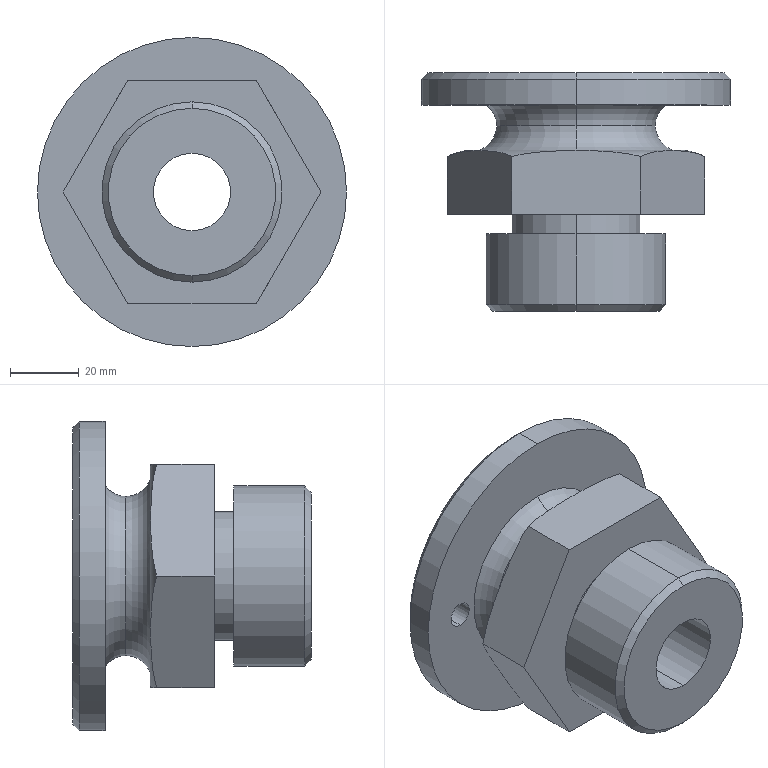Part | SolidWorks | features Chamfer 2, ICE 2, RevCut 1, Revolution 1, Scale 1 | 1 solid | 34 faces | box 90 x 69.375 x 90 mm | volume 178103 mm3 | cylinder 12 | plane 12 | torus 6 | cone 4 | commonest cylinder face diameters 7.5 x4 22.5 x2 37.5 x2 52.5 x2 90 x2
STEP:
#1=CARTESIAN_POINT('',(0.,27.536,-28.125));
#2=VERTEX_POINT('',#1);
#3=CARTESIAN_POINT('',(0.,34.594,-23.16));
#4=VERTEX_POINT('',#3);
#5=CARTESIAN_POINT('',(0.,34.594,-30.66));
#6=DIRECTION('',(-1.,0.,0.));
#7=DIRECTION('',(0.,0.,1.));
#8=AXIS2_PLACEMENT_3D('',#5,#6,#7);
#9=CIRCLE('',#8,7.5);
#10=EDGE_CURVE('',#2,#4,#9,.T.);
#11=ORIENTED_EDGE('',*,*,#10,.T.);
#12=CARTESIAN_POINT('',(0.,34.594,23.16));
#13=VERTEX_POINT('',#12);
#14=CARTESIAN_POINT('',(0.,34.594,-0.000000001));
#15=DIRECTION('',(0.,-1.,0.));
#16=DIRECTION('',(0.,0.,-1.));
#17=AXIS2_PLACEMENT_3D('',#14,#15,#16);
#18=CIRCLE('',#17,23.16);
#19=EDGE_CURVE('',#4,#13,#18,.T.);
#20=ORIENTED_EDGE('',*,*,#19,.T.);
#21=CARTESIAN_POINT('',(0.,27.536,28.125));
#22=VERTEX_POINT('',#21);
#23=CARTESIAN_POINT('',(0.,34.594,30.66));
#24=DIRECTION('',(1.,0.,0.));
#25=DIRECTION('',(0.,0.,-1.));
#26=AXIS2_PLACEMENT_3D('',#23,#24,#25);
#27=CIRCLE('',#26,7.5);
#28=EDGE_CURVE('',#22,#13,#27,.T.);
#29=ORIENTED_EDGE('',*,*,#28,.F.);
#30=CARTESIAN_POINT('',(0.,27.536,-0.000000001));
#31=DIRECTION('',(0.,-1.,0.));
#32=DIRECTION('',(0.,0.,-1.));
#33=AXIS2_PLACEMENT_3D('',#30,#31,#32);
#34=CIRCLE('',#33,28.125);
#35=EDGE_CURVE('',#2,#22,#34,.T.);
#36=ORIENTED_EDGE('',*,*,#35,.F.);
#37=EDGE_LOOP('',(#11,#20,#29,#36));
#38=FACE_OUTER_BOUND('',#37,.T.);
#39=CARTESIAN_POINT('',(0.,34.594,-0.000000001));
#40=DIRECTION('',(0.,-1.,0.));
#41=DIRECTION('',(0.,0.,-1.));
#42=AXIS2_PLACEMENT_3D('',#39,#40,#41);
#43=TOROIDAL_SURFACE('',#42,30.66,7.5);
#44=ADVANCED_FACE('',(#38),#43,.F.);
#45=ORIENTED_EDGE('',*,*,#28,.T.);
#46=CARTESIAN_POINT('',(0.,34.594,-0.000000001));
#47=DIRECTION('',(0.,-1.,0.));
#48=DIRECTION('',(0.,0.,-1.));
#49=AXIS2_PLACEMENT_3D('',#46,#47,#48);
#50=CIRCLE('',#49,23.16);
#51=EDGE_CURVE('',#13,#4,#50,.T.);
#52=ORIENTED_EDGE('',*,*,#51,.T.);
#53=ORIENTED_EDGE('',*,*,#10,.F.);
#54=CARTESIAN_POINT('',(0.,27.536,-0.000000001));
#55=DIRECTION('',(0.,-1.,0.));
#56=DIRECTION('',(0.,0.,-1.));
#57=AXIS2_PLACEMENT_3D('',#54,#55,#56);
#58=CIRCLE('',#57,28.125);
#59=EDGE_CURVE('',#22,#2,#58,.T.);
#60=ORIENTED_EDGE('',*,*,#59,.F.);
#61=EDGE_LOOP('',(#45,#52,#53,#60));
#62=FACE_OUTER_BOUND('',#61,.T.);
#63=CARTESIAN_POINT('',(0.,34.594,-0.000000001));
#64=DIRECTION('',(0.,-1.,0.));
#65=DIRECTION('',(0.,0.,-1.));
#66=AXIS2_PLACEMENT_3D('',#63,#64,#65);
#67=TOROIDAL_SURFACE('',#66,30.66,7.5);
#68=ADVANCED_FACE('',(#62),#67,.F.);
#69=CARTESIAN_POINT('',(-31.875,40.661,-3.75));
#70=VERTEX_POINT('',#69);
#71=CARTESIAN_POINT('',(-31.875,40.661,3.75));
#72=VERTEX_POINT('',#71);
#73=CARTESIAN_POINT('',(-31.875,40.661,-0.000000001));
#74=DIRECTION('',(0.,1.,0.));
#75=DIRECTION('',(0.,0.,-1.));
#76=AXIS2_PLACEMENT_3D('',#73,#74,#75);
#77=CIRCLE('',#76,3.75);
#78=EDGE_CURVE('',#70,#72,#77,.T.);
#79=ORIENTED_EDGE('',*,*,#78,.F.);
#80=CARTESIAN_POINT('',(-31.875,50.036,-3.75));
#81=VERTEX_POINT('',#80);
#82=CARTESIAN_POINT('',(-31.875,-19.341,-3.75));
#83=DIRECTION('',(0.,1.,0.));
#84=VECTOR('',#83,1000.);
#85=LINE('',#82,#84);
#86=EDGE_CURVE('',#70,#81,#85,.T.);
#87=ORIENTED_EDGE('',*,*,#86,.T.);
#88=CARTESIAN_POINT('',(-31.875,50.036,3.75));
#89=VERTEX_POINT('',#88);
#90=CARTESIAN_POINT('',(-31.875,50.036,-0.000000001));
#91=DIRECTION('',(0.,1.,0.));
#92=DIRECTION('',(0.,0.,-1.));
#93=AXIS2_PLACEMENT_3D('',#90,#91,#92);
#94=CIRCLE('',#93,3.75);
#95=EDGE_CURVE('',#81,#89,#94,.T.);
#96=ORIENTED_EDGE('',*,*,#95,.T.);
#97=CARTESIAN_POINT('',(-31.875,-19.341,3.75));
#98=DIRECTION('',(0.,1.,0.));
#99=VECTOR('',#98,1000.);
#100=LINE('',#97,#99);
#101=EDGE_CURVE('',#72,#89,#100,.T.);
#102=ORIENTED_EDGE('',*,*,#101,.F.);
#103=EDGE_LOOP('',(#79,#87,#96,#102));
#104=FACE_OUTER_BOUND('',#103,.T.);
#105=CARTESIAN_POINT('',(-31.875,-19.341,-0.000000001));
#106=DIRECTION('',(0.,1.,0.));
#107=DIRECTION('',(0.,0.,1.));
#108=AXIS2_PLACEMENT_3D('',#105,#106,#107);
#109=CYLINDRICAL_SURFACE('',#108,3.75);
#110=ADVANCED_FACE('',(#104),#109,.F.);
#111=CARTESIAN_POINT('',(31.875,40.661,-3.75));
#112=VERTEX_POINT('',#111);
#113=CARTESIAN_POINT('',(31.875,40.661,3.75));
#114=VERTEX_POINT('',#113);
#115=CARTESIAN_POINT('',(31.875,40.661,-0.000000001));
#116=DIRECTION('',(0.,1.,0.));
#117=DIRECTION('',(0.,0.,-1.));
#118=AXIS2_PLACEMENT_3D('',#115,#116,#117);
#119=CIRCLE('',#118,3.75);
#120=EDGE_CURVE('',#112,#114,#119,.T.);
#121=ORIENTED_EDGE('',*,*,#120,.F.);
#122=CARTESIAN_POINT('',(31.875,50.036,-3.75));
#123=VERTEX_POINT('',#122);
#124=CARTESIAN_POINT('',(31.875,-19.341,-3.75));
#125=DIRECTION('',(0.,1.,0.));
#126=VECTOR('',#125,1000.);
#127=LINE('',#124,#126);
#128=EDGE_CURVE('',#112,#123,#127,.T.);
#129=ORIENTED_EDGE('',*,*,#128,.T.);
#130=CARTESIAN_POINT('',(31.875,50.036,3.75));
#131=VERTEX_POINT('',#130);
#132=CARTESIAN_POINT('',(31.875,50.036,-0.000000001));
#133=DIRECTION('',(0.,1.,0.));
#134=DIRECTION('',(0.,0.,1.));
#135=AXIS2_PLACEMENT_3D('',#132,#133,#134);
#136=CIRCLE('',#135,3.75);
#137=EDGE_CURVE('',#123,#131,#136,.T.);
#138=ORIENTED_EDGE('',*,*,#137,.T.);
#139=CARTESIAN_POINT('',(31.875,-19.341,3.75));
#140=DIRECTION('',(0.,1.,0.));
#141=VECTOR('',#140,1000.);
#142=LINE('',#139,#141);
#143=EDGE_CURVE('',#114,#131,#142,.T.);
#144=ORIENTED_EDGE('',*,*,#143,.F.);
#145=EDGE_LOOP('',(#121,#129,#138,#144));
#146=FACE_OUTER_BOUND('',#145,.T.);
#147=CARTESIAN_POINT('',(31.875,-19.341,-0.000000001));
#148=DIRECTION('',(0.,1.,0.));
#149=DIRECTION('',(0.,0.,1.));
#150=AXIS2_PLACEMENT_3D('',#147,#148,#149);
#151=CYLINDRICAL_SURFACE('',#150,3.75);
#152=ADVANCED_FACE('',(#146),#151,.F.);
#153=CARTESIAN_POINT('',(0.,50.036,43.125));
#154=VERTEX_POINT('',#153);
#155=CARTESIAN_POINT('',(0.,50.036,-43.125));
#156=VERTEX_POINT('',#155);
#157=CARTESIAN_POINT('',(0.,50.036,-0.000000001));
#158=DIRECTION('',(0.,1.,0.));
#159=DIRECTION('',(0.,0.,1.));
#160=AXIS2_PLACEMENT_3D('',#157,#158,#159);
#161=CIRCLE('',#160,43.125);
#162=EDGE_CURVE('',#154,#156,#161,.T.);
#163=ORIENTED_EDGE('',*,*,#162,.F.);
#164=CARTESIAN_POINT('',(0.,48.161,45.));
#165=VERTEX_POINT('',#164);
#166=CARTESIAN_POINT('',(0.,48.161,45.));
#167=DIRECTION('',(0.,-0.7071,0.7071));
#168=VECTOR('',#167,1000.);
#169=LINE('',#166,#168);
#170=EDGE_CURVE('',#154,#165,#169,.T.);
#171=ORIENTED_EDGE('',*,*,#170,.T.);
#172=CARTESIAN_POINT('',(0.,48.161,-45.));
#173=VERTEX_POINT('',#172);
#174=CARTESIAN_POINT('',(0.,48.161,-0.000000001));
#175=DIRECTION('',(0.,-1.,0.));
#176=DIRECTION('',(0.,0.,1.));
#177=AXIS2_PLACEMENT_3D('',#174,#175,#176);
#178=CIRCLE('',#177,45.);
#179=EDGE_CURVE('',#173,#165,#178,.T.);
#180=ORIENTED_EDGE('',*,*,#179,.F.);
#181=CARTESIAN_POINT('',(0.,48.161,-45.));
#182=DIRECTION('',(0.,-0.7071,-0.7071));
#183=VECTOR('',#182,1000.);
#184=LINE('',#181,#183);
#185=EDGE_CURVE('',#156,#173,#184,.T.);
#186=ORIENTED_EDGE('',*,*,#185,.F.);
#187=EDGE_LOOP('',(#163,#171,#180,#186));
#188=FACE_OUTER_BOUND('',#187,.T.);
#189=CARTESIAN_POINT('',(0.,48.161,-0.000000001));
#190=DIRECTION('',(0.,-1.,0.));
#191=DIRECTION('',(0.,0.,-1.));
#192=AXIS2_PLACEMENT_3D('',#189,#190,#191);
#193=CONICAL_SURFACE('',#192,45.,0.7854);
#194=ADVANCED_FACE('',(#188),#193,.T.);
#195=CARTESIAN_POINT('',(0.,27.536,-31.152));
#196=VERTEX_POINT('',#195);
#197=CARTESIAN_POINT('',(0.,27.536,31.152));
#198=VERTEX_POINT('',#197);
#199=CARTESIAN_POINT('',(0.,27.536,-0.000000001));
#200=DIRECTION('',(0.,-1.,0.));
#201=DIRECTION('',(0.,0.,-1.));
#202=AXIS2_PLACEMENT_3D('',#199,#200,#201);
#203=CIRCLE('',#202,31.152);
#204=EDGE_CURVE('',#196,#198,#203,.T.);
#205=ORIENTED_EDGE('',*,*,#204,.T.);
#206=CARTESIAN_POINT('',(0.,27.363,32.476));
#207=VERTEX_POINT('',#206);
#208=CARTESIAN_POINT('',(0.,10.729,29.639));
#209=DIRECTION('',(1.,0.,0.));
#210=DIRECTION('',(0.,0.,-1.));
#211=AXIS2_PLACEMENT_3D('',#208,#209,#210);
#212=CIRCLE('',#211,16.875);
#213=EDGE_CURVE('',#198,#207,#212,.T.);
#214=ORIENTED_EDGE('',*,*,#213,.T.);
#215=CARTESIAN_POINT('',(18.75,25.661,32.476));
#216=VERTEX_POINT('',#215);
#217=CARTESIAN_POINT('',(18.75,25.661,32.476));
#218=CARTESIAN_POINT('',(17.221,26.063,32.476));
#219=CARTESIAN_POINT('',(15.679,26.359,32.476));
#220=CARTESIAN_POINT('',(12.575,26.81,32.476));
#221=CARTESIAN_POINT('',(11.014,26.965,32.476));
#222=CARTESIAN_POINT('',(7.88,27.189,32.476));
#223=CARTESIAN_POINT('',(6.307,27.258,32.476));
#224=CARTESIAN_POINT('',(3.943,27.323,32.476));
#225=CARTESIAN_POINT('',(3.155,27.338,32.476));
#226=CARTESIAN_POINT('',(1.972,27.354,32.476));
#227=CARTESIAN_POINT('',(1.577,27.357,32.476));
#228=CARTESIAN_POINT('',(0.9859,27.361,32.476));
#229=CARTESIAN_POINT('',(0.7887,27.362,32.476));
#230=CARTESIAN_POINT('',(0.3944,27.363,32.476));
#231=CARTESIAN_POINT('',(0.1986,27.363,32.476));
#232=CARTESIAN_POINT('',(0.,27.363,32.476));
#233=B_SPLINE_CURVE_WITH_KNOTS('',3,(#217,#218,#219,#220,#221,#222,#223,#224,#225,#226,#227,#228,#229,#230,#231,#232),.UNSPECIFIED.,.F.,.F.,(4,2,2,2,2,2,2,4),(0.1464,0.1511,0.1559,0.1607,0.163,0.1642,0.1648,0.1654),.UNSPECIFIED.);
#234=EDGE_CURVE('',#216,#207,#233,.T.);
#235=ORIENTED_EDGE('',*,*,#234,.F.);
#236=CARTESIAN_POINT('',(37.5,25.661,-0.000000001));
#237=VERTEX_POINT('',#236);
#238=CARTESIAN_POINT('',(37.5,25.661,-0.000000001));
#239=CARTESIAN_POINT('',(36.729,26.067,1.336));
#240=CARTESIAN_POINT('',(35.953,26.363,2.679));
#241=CARTESIAN_POINT('',(34.397,26.813,5.375));
#242=CARTESIAN_POINT('',(33.616,26.968,6.727));
#243=CARTESIAN_POINT('',(32.052,27.19,9.437));
#244=CARTESIAN_POINT('',(31.268,27.258,10.795));
#245=CARTESIAN_POINT('',(29.698,27.345,13.513));
#246=CARTESIAN_POINT('',(28.912,27.363,14.874));
#247=CARTESIAN_POINT('',(27.339,27.363,17.599));
#248=CARTESIAN_POINT('',(26.551,27.345,18.963));
#249=CARTESIAN_POINT('',(24.977,27.258,21.69));
#250=CARTESIAN_POINT('',(24.192,27.19,23.051));
#251=CARTESIAN_POINT('',(22.625,26.966,25.764));
#252=CARTESIAN_POINT('',(21.844,26.811,27.117));
#253=CARTESIAN_POINT('',(20.29,26.36,29.808));
#254=CARTESIAN_POINT('',(19.517,26.065,31.147));
#255=CARTESIAN_POINT('',(18.75,25.661,32.476));
#256=B_SPLINE_CURVE_WITH_KNOTS('',3,(#238,#239,#240,#241,#242,#243,#244,#245,#246,#247,#248,#249,#250,#251,#252,#253,#254,#255),.UNSPECIFIED.,.F.,.F.,(4,2,2,2,2,2,2,2,4),(0.00000044,0.004706,0.009412,0.01412,0.01882,0.02353,0.02824,0.03294,0.03765),.UNSPECIFIED.);
#257=EDGE_CURVE('',#237,#216,#256,.T.);
#258=ORIENTED_EDGE('',*,*,#257,.F.);
#259=CARTESIAN_POINT('',(18.75,25.661,-32.476));
#260=VERTEX_POINT('',#259);
#261=CARTESIAN_POINT('',(18.75,25.661,-32.476));
#262=CARTESIAN_POINT('',(19.521,26.067,-31.14));
#263=CARTESIAN_POINT('',(20.297,26.363,-29.797));
#264=CARTESIAN_POINT('',(21.853,26.813,-27.101));
#265=CARTESIAN_POINT('',(22.634,26.968,-25.749));
#266=CARTESIAN_POINT('',(24.198,27.19,-23.039));
#267=CARTESIAN_POINT('',(24.982,27.258,-21.681));
#268=CARTESIAN_POINT('',(26.552,27.345,-18.963));
#269=CARTESIAN_POINT('',(27.338,27.363,-17.602));
#270=CARTESIAN_POINT('',(28.911,27.363,-14.877));
#271=CARTESIAN_POINT('',(29.699,27.345,-13.513));
#272=CARTESIAN_POINT('',(31.273,27.258,-10.786));
#273=CARTESIAN_POINT('',(32.058,27.19,-9.425));
#274=CARTESIAN_POINT('',(33.625,26.966,-6.712));
#275=CARTESIAN_POINT('',(34.406,26.811,-5.359));
#276=CARTESIAN_POINT('',(35.96,26.36,-2.668));
#277=CARTESIAN_POINT('',(36.733,26.065,-1.329));
#278=CARTESIAN_POINT('',(37.5,25.661,-0.000000001));
#279=B_SPLINE_CURVE_WITH_KNOTS('',3,(#261,#262,#263,#264,#265,#266,#267,#268,#269,#270,#271,#272,#273,#274,#275,#276,#277,#278),.UNSPECIFIED.,.F.,.F.,(4,2,2,2,2,2,2,2,4),(0.00000044,0.004706,0.009412,0.01412,0.01882,0.02353,0.02824,0.03294,0.03765),.UNSPECIFIED.);
#280=EDGE_CURVE('',#260,#237,#279,.T.);
#281=ORIENTED_EDGE('',*,*,#280,.F.);
#282=CARTESIAN_POINT('',(0.,27.363,-32.476));
#283=VERTEX_POINT('',#282);
#284=CARTESIAN_POINT('',(0.,27.363,-32.476));
#285=CARTESIAN_POINT('',(1.575,27.363,-32.476));
#286=CARTESIAN_POINT('',(3.148,27.345,-32.476));
#287=CARTESIAN_POINT('',(6.292,27.258,-32.476));
#288=CARTESIAN_POINT('',(7.863,27.19,-32.476));
#289=CARTESIAN_POINT('',(10.999,26.966,-32.476));
#290=CARTESIAN_POINT('',(12.565,26.811,-32.476));
#291=CARTESIAN_POINT('',(15.689,26.357,-32.476));
#292=CARTESIAN_POINT('',(17.234,26.06,-32.476));
#293=CARTESIAN_POINT('',(18.75,25.661,-32.476));
#294=B_SPLINE_CURVE_WITH_KNOTS('',3,(#284,#285,#286,#287,#288,#289,#290,#291,#292,#293),.UNSPECIFIED.,.F.,.F.,(4,2,2,2,4),(0.,0.004716,0.009432,0.01415,0.01886),.UNSPECIFIED.);
#295=EDGE_CURVE('',#283,#260,#294,.T.);
#296=ORIENTED_EDGE('',*,*,#295,.F.);
#297=CARTESIAN_POINT('',(0.,10.729,-29.639));
#298=DIRECTION('',(-1.,0.,0.));
#299=DIRECTION('',(0.,0.,1.));
#300=AXIS2_PLACEMENT_3D('',#297,#298,#299);
#301=CIRCLE('',#300,16.875);
#302=EDGE_CURVE('',#196,#283,#301,.T.);
#303=ORIENTED_EDGE('',*,*,#302,.F.);
#304=EDGE_LOOP('',(#205,#214,#235,#258,#281,#296,#303));
#305=FACE_OUTER_BOUND('',#304,.T.);
#306=CARTESIAN_POINT('',(0.,10.729,-0.000000001));
#307=DIRECTION('',(0.,-1.,0.));
#308=DIRECTION('',(0.,0.,-1.));
#309=AXIS2_PLACEMENT_3D('',#306,#307,#308);
#310=TOROIDAL_SURFACE('',#309,29.639,16.875);
#311=ADVANCED_FACE('',(#305),#310,.T.);
#312=CARTESIAN_POINT('',(0.,-19.339,-24.375));
#313=VERTEX_POINT('',#312);
#314=CARTESIAN_POINT('',(0.,-19.339,24.375));
#315=VERTEX_POINT('',#314);
#316=CARTESIAN_POINT('',(0.,-19.339,-0.000000001));
#317=DIRECTION('',(0.,-1.,0.));
#318=DIRECTION('',(0.,0.,-1.));
#319=AXIS2_PLACEMENT_3D('',#316,#317,#318);
#320=CIRCLE('',#319,24.375);
#321=EDGE_CURVE('',#313,#315,#320,.T.);
#322=ORIENTED_EDGE('',*,*,#321,.F.);
#323=CARTESIAN_POINT('',(0.,-17.464,-26.25));
#324=VERTEX_POINT('',#323);
#325=CARTESIAN_POINT('',(0.,-19.339,-24.375));
#326=DIRECTION('',(0.,0.7071,-0.7071));
#327=VECTOR('',#326,1000.);
#328=LINE('',#325,#327);
#329=EDGE_CURVE('',#313,#324,#328,.T.);
#330=ORIENTED_EDGE('',*,*,#329,.T.);
#331=CARTESIAN_POINT('',(0.,-17.464,26.25));
#332=VERTEX_POINT('',#331);
#333=CARTESIAN_POINT('',(0.,-17.464,-0.000000001));
#334=DIRECTION('',(0.,1.,0.));
#335=DIRECTION('',(0.,0.,-1.));
#336=AXIS2_PLACEMENT_3D('',#333,#334,#335);
#337=CIRCLE('',#336,26.25);
#338=EDGE_CURVE('',#332,#324,#337,.T.);
#339=ORIENTED_EDGE('',*,*,#338,.F.);
#340=CARTESIAN_POINT('',(0.,-19.339,24.375));
#341=DIRECTION('',(0.,0.7071,0.7071));
#342=VECTOR('',#341,1000.);
#343=LINE('',#340,#342);
#344=EDGE_CURVE('',#315,#332,#343,.T.);
#345=ORIENTED_EDGE('',*,*,#344,.F.);
#346=EDGE_LOOP('',(#322,#330,#339,#345));
#347=FACE_OUTER_BOUND('',#346,.T.);
#348=CARTESIAN_POINT('',(0.,-19.339,-0.000000001));
#349=DIRECTION('',(0.,1.,0.));
#350=DIRECTION('',(0.,0.,1.));
#351=AXIS2_PLACEMENT_3D('',#348,#349,#350);
#352=CONICAL_SURFACE('',#351,24.375,0.7854);
#353=ADVANCED_FACE('',(#347),#352,.T.);
#354=CARTESIAN_POINT('',(0.,50.036,11.25));
#355=VERTEX_POINT('',#354);
#356=CARTESIAN_POINT('',(0.,50.036,-11.25));
#357=VERTEX_POINT('',#356);
#358=CARTESIAN_POINT('',(0.,50.036,-0.000000001));
#359=DIRECTION('',(0.,-1.,0.));
#360=DIRECTION('',(0.,0.,-1.));
#361=AXIS2_PLACEMENT_3D('',#358,#359,#360);
#362=CIRCLE('',#361,11.25);
#363=EDGE_CURVE('',#355,#357,#362,.T.);
#364=ORIENTED_EDGE('',*,*,#363,.F.);
#365=CARTESIAN_POINT('',(0.,-19.339,11.25));
#366=VERTEX_POINT('',#365);
#367=CARTESIAN_POINT('',(0.,-19.339,11.25));
#368=DIRECTION('',(0.,-1.,0.));
#369=VECTOR('',#368,1000.);
#370=LINE('',#367,#369);
#371=EDGE_CURVE('',#355,#366,#370,.T.);
#372=ORIENTED_EDGE('',*,*,#371,.T.);
#373=CARTESIAN_POINT('',(0.,-19.339,-11.25));
#374=VERTEX_POINT('',#373);
#375=CARTESIAN_POINT('',(0.,-19.339,-0.000000001));
#376=DIRECTION('',(0.,-1.,0.));
#377=DIRECTION('',(0.,0.,-1.));
#378=AXIS2_PLACEMENT_3D('',#375,#376,#377);
#379=CIRCLE('',#378,11.25);
#380=EDGE_CURVE('',#366,#374,#379,.T.);
#381=ORIENTED_EDGE('',*,*,#380,.T.);
#382=CARTESIAN_POINT('',(0.,-19.339,-11.25));
#383=DIRECTION('',(0.,-1.,0.));
#384=VECTOR('',#383,1000.);
#385=LINE('',#382,#384);
#386=EDGE_CURVE('',#357,#374,#385,.T.);
#387=ORIENTED_EDGE('',*,*,#386,.F.);
#388=EDGE_LOOP('',(#364,#372,#381,#387));
#389=FACE_OUTER_BOUND('',#388,.T.);
#390=CARTESIAN_POINT('',(0.,-19.339,-0.000000001));
#391=DIRECTION('',(0.,-1.,0.));
#392=DIRECTION('',(0.,0.,-1.));
#393=AXIS2_PLACEMENT_3D('',#390,#391,#392);
#394=CYLINDRICAL_SURFACE('',#393,11.25);
#395=ADVANCED_FACE('',(#389),#394,.F.);
#396=ORIENTED_EDGE('',*,*,#179,.T.);
#397=CARTESIAN_POINT('',(0.,40.661,45.));
#398=VERTEX_POINT('',#397);
#399=CARTESIAN_POINT('',(0.,-19.339,45.));
#400=DIRECTION('',(0.,-1.,0.));
#401=VECTOR('',#400,1000.);
#402=LINE('',#399,#401);
#403=EDGE_CURVE('',#165,#398,#402,.T.);
#404=ORIENTED_EDGE('',*,*,#403,.T.);
#405=CARTESIAN_POINT('',(0.,40.661,-45.));
#406=VERTEX_POINT('',#405);
#407=CARTESIAN_POINT('',(0.,40.661,-0.000000001));
#408=DIRECTION('',(0.,-1.,0.));
#409=DIRECTION('',(0.,0.,-1.));
#410=AXIS2_PLACEMENT_3D('',#407,#408,#409);
#411=CIRCLE('',#410,45.);
#412=EDGE_CURVE('',#406,#398,#411,.T.);
#413=ORIENTED_EDGE('',*,*,#412,.F.);
#414=CARTESIAN_POINT('',(0.,-19.339,-45.));
#415=DIRECTION('',(0.,-1.,0.));
#416=VECTOR('',#415,1000.);
#417=LINE('',#414,#416);
#418=EDGE_CURVE('',#173,#406,#417,.T.);
#419=ORIENTED_EDGE('',*,*,#418,.F.);
#420=EDGE_LOOP('',(#396,#404,#413,#419));
#421=FACE_OUTER_BOUND('',#420,.T.);
#422=CARTESIAN_POINT('',(0.,-19.339,-0.000000001));
#423=DIRECTION('',(0.,-1.,0.));
#424=DIRECTION('',(0.,0.,-1.));
#425=AXIS2_PLACEMENT_3D('',#422,#423,#424);
#426=CYLINDRICAL_SURFACE('',#425,45.);
#427=ADVANCED_FACE('',(#421),#426,.T.);
#428=ORIENTED_EDGE('',*,*,#51,.F.);
#429=CARTESIAN_POINT('',(0.,40.661,26.25));
#430=VERTEX_POINT('',#429);
#431=CARTESIAN_POINT('',(0.,34.594,30.66));
#432=DIRECTION('',(1.,0.,0.));
#433=DIRECTION('',(0.,0.,-1.));
#434=AXIS2_PLACEMENT_3D('',#431,#432,#433);
#435=CIRCLE('',#434,7.5);
#436=EDGE_CURVE('',#13,#430,#435,.T.);
#437=ORIENTED_EDGE('',*,*,#436,.T.);
#438=CARTESIAN_POINT('',(0.,40.661,-26.25));
#439=VERTEX_POINT('',#438);
#440=CARTESIAN_POINT('',(0.,40.661,-0.000000001));
#441=DIRECTION('',(0.,-1.,0.));
#442=DIRECTION('',(0.,0.,-1.));
#443=AXIS2_PLACEMENT_3D('',#440,#441,#442);
#444=CIRCLE('',#443,26.25);
#445=EDGE_CURVE('',#430,#439,#444,.T.);
#446=ORIENTED_EDGE('',*,*,#445,.T.);
#447=CARTESIAN_POINT('',(0.,34.594,-30.66));
#448=DIRECTION('',(-1.,0.,0.));
#449=DIRECTION('',(0.,0.,1.));
#450=AXIS2_PLACEMENT_3D('',#447,#448,#449);
#451=CIRCLE('',#450,7.5);
#452=EDGE_CURVE('',#4,#439,#451,.T.);
#453=ORIENTED_EDGE('',*,*,#452,.F.);
#454=EDGE_LOOP('',(#428,#437,#446,#453));
#455=FACE_OUTER_BOUND('',#454,.T.);
#456=CARTESIAN_POINT('',(0.,34.594,-0.000000001));
#457=DIRECTION('',(0.,-1.,0.));
#458=DIRECTION('',(0.,0.,-1.));
#459=AXIS2_PLACEMENT_3D('',#456,#457,#458);
#460=TOROIDAL_SURFACE('',#459,30.66,7.5);
#461=ADVANCED_FACE('',(#455),#460,.F.);
#462=CARTESIAN_POINT('',(0.,8.786,-18.75));
#463=VERTEX_POINT('',#462);
#464=CARTESIAN_POINT('',(0.,8.786,18.75));
#465=VERTEX_POINT('',#464);
#466=CARTESIAN_POINT('',(0.,8.786,-0.000000001));
#467=DIRECTION('',(0.,-1.,0.));
#468=DIRECTION('',(0.,0.,-1.));
#469=AXIS2_PLACEMENT_3D('',#466,#467,#468);
#470=CIRCLE('',#469,18.75);
#471=EDGE_CURVE('',#463,#465,#470,.T.);
#472=ORIENTED_EDGE('',*,*,#471,.T.);
#473=CARTESIAN_POINT('',(0.,3.161,18.75));
#474=VERTEX_POINT('',#473);
#475=CARTESIAN_POINT('',(0.,-19.339,18.75));
#476=DIRECTION('',(0.,-1.,0.));
#477=VECTOR('',#476,1000.);
#478=LINE('',#475,#477);
#479=EDGE_CURVE('',#465,#474,#478,.T.);
#480=ORIENTED_EDGE('',*,*,#479,.T.);
#481=CARTESIAN_POINT('',(0.,3.161,-18.75));
#482=VERTEX_POINT('',#481);
#483=CARTESIAN_POINT('',(0.,3.161,-0.000000001));
#484=DIRECTION('',(0.,-1.,0.));
#485=DIRECTION('',(0.,0.,-1.));
#486=AXIS2_PLACEMENT_3D('',#483,#484,#485);
#487=CIRCLE('',#486,18.75);
#488=EDGE_CURVE('',#482,#474,#487,.T.);
#489=ORIENTED_EDGE('',*,*,#488,.F.);
#490=CARTESIAN_POINT('',(0.,-19.339,-18.75));
#491=DIRECTION('',(0.,-1.,0.));
#492=VECTOR('',#491,1000.);
#493=LINE('',#490,#492);
#494=EDGE_CURVE('',#463,#482,#493,.T.);
#495=ORIENTED_EDGE('',*,*,#494,.F.);
#496=EDGE_LOOP('',(#472,#480,#489,#495));
#497=FACE_OUTER_BOUND('',#496,.T.);
#498=CARTESIAN_POINT('',(0.,-19.339,-0.000000001));
#499=DIRECTION('',(0.,-1.,0.));
#500=DIRECTION('',(0.,0.,-1.));
#501=AXIS2_PLACEMENT_3D('',#498,#499,#500);
#502=CYLINDRICAL_SURFACE('',#501,18.75);
#503=ADVANCED_FACE('',(#497),#502,.T.);
#504=CARTESIAN_POINT('',(0.,3.161,-26.25));
#505=VERTEX_POINT('',#504);
#506=CARTESIAN_POINT('',(0.,3.161,26.25));
#507=VERTEX_POINT('',#506);
#508=CARTESIAN_POINT('',(0.,3.161,-0.000000001));
#509=DIRECTION('',(0.,-1.,0.));
#510=DIRECTION('',(0.,0.,-1.));
#511=AXIS2_PLACEMENT_3D('',#508,#509,#510);
#512=CIRCLE('',#511,26.25);
#513=EDGE_CURVE('',#505,#507,#512,.T.);
#514=ORIENTED_EDGE('',*,*,#513,.T.);
#515=CARTESIAN_POINT('',(0.,-19.339,26.25));
#516=DIRECTION('',(0.,-1.,0.));
#517=VECTOR('',#516,1000.);
#518=LINE('',#515,#517);
#519=EDGE_CURVE('',#507,#332,#518,.T.);
#520=ORIENTED_EDGE('',*,*,#519,.T.);
#521=ORIENTED_EDGE('',*,*,#338,.T.);
#522=CARTESIAN_POINT('',(0.,-19.339,-26.25));
#523=DIRECTION('',(0.,-1.,0.));
#524=VECTOR('',#523,1000.);
#525=LINE('',#522,#524);
#526=EDGE_CURVE('',#505,#324,#525,.T.);
#527=ORIENTED_EDGE('',*,*,#526,.F.);
#528=EDGE_LOOP('',(#514,#520,#521,#527));
#529=FACE_OUTER_BOUND('',#528,.T.);
#530=CARTESIAN_POINT('',(0.,-19.339,-0.000000001));
#531=DIRECTION('',(0.,-1.,0.));
#532=DIRECTION('',(0.,0.,-1.));
#533=AXIS2_PLACEMENT_3D('',#530,#531,#532);
#534=CYLINDRICAL_SURFACE('',#533,26.25);
#535=ADVANCED_FACE('',(#529),#534,.T.);
#536=ORIENTED_EDGE('',*,*,#35,.T.);
#537=ORIENTED_EDGE('',*,*,#59,.T.);
#538=EDGE_LOOP('',(#536,#537));
#539=FACE_BOUND('',#538,.T.);
#540=ORIENTED_EDGE('',*,*,#204,.F.);
#541=CARTESIAN_POINT('',(0.,27.536,-0.000000001));
#542=DIRECTION('',(0.,-1.,0.));
#543=DIRECTION('',(0.,0.,-1.));
#544=AXIS2_PLACEMENT_3D('',#541,#542,#543);
#545=CIRCLE('',#544,31.152);
#546=EDGE_CURVE('',#198,#196,#545,.T.);
#547=ORIENTED_EDGE('',*,*,#546,.F.);
#548=EDGE_LOOP('',(#540,#547));
#549=FACE_OUTER_BOUND('',#548,.T.);
#550=CARTESIAN_POINT('',(37.5,27.536,-0.000000001));
#551=DIRECTION('',(0.,1.,0.));
#552=DIRECTION('',(0.,0.,1.));
#553=AXIS2_PLACEMENT_3D('',#550,#551,#552);
#554=PLANE('',#553);
#555=ADVANCED_FACE('',(#539,#549),#554,.T.);
#556=CARTESIAN_POINT('',(-18.75,8.786,32.476));
#557=VERTEX_POINT('',#556);
#558=CARTESIAN_POINT('',(-18.75,25.661,32.476));
#559=VERTEX_POINT('',#558);
#560=CARTESIAN_POINT('',(-18.75,-19.339,32.476));
#561=DIRECTION('',(0.,1.,0.));
#562=VECTOR('',#561,1000.);
#563=LINE('',#560,#562);
#564=EDGE_CURVE('',#557,#559,#563,.T.);
#565=ORIENTED_EDGE('',*,*,#564,.T.);
#566=CARTESIAN_POINT('',(-37.5,25.661,-0.000000001));
#567=VERTEX_POINT('',#566);
#568=CARTESIAN_POINT('',(-18.75,25.661,32.476));
#569=CARTESIAN_POINT('',(-19.521,26.067,31.14));
#570=CARTESIAN_POINT('',(-20.297,26.363,29.797));
#571=CARTESIAN_POINT('',(-21.853,26.813,27.101));
#572=CARTESIAN_POINT('',(-22.634,26.968,25.749));
#573=CARTESIAN_POINT('',(-24.198,27.19,23.039));
#574=CARTESIAN_POINT('',(-24.982,27.258,21.681));
#575=CARTESIAN_POINT('',(-26.552,27.345,18.963));
#576=CARTESIAN_POINT('',(-27.338,27.363,17.602));
#577=CARTESIAN_POINT('',(-28.911,27.363,14.877));
#578=CARTESIAN_POINT('',(-29.699,27.345,13.513));
#579=CARTESIAN_POINT('',(-31.273,27.258,10.786));
#580=CARTESIAN_POINT('',(-32.058,27.19,9.425));
#581=CARTESIAN_POINT('',(-33.625,26.966,6.712));
#582=CARTESIAN_POINT('',(-34.406,26.811,5.359));
#583=CARTESIAN_POINT('',(-35.96,26.36,2.668));
#584=CARTESIAN_POINT('',(-36.733,26.065,1.329));
#585=CARTESIAN_POINT('',(-37.5,25.661,-0.000000001));
#586=B_SPLINE_CURVE_WITH_KNOTS('',3,(#568,#569,#570,#571,#572,#573,#574,#575,#576,#577,#578,#579,#580,#581,#582,#583,#584,#585),.UNSPECIFIED.,.F.,.F.,(4,2,2,2,2,2,2,2,4),(0.00000044,0.004706,0.009412,0.01412,0.01882,0.02353,0.02824,0.03294,0.03765),.UNSPECIFIED.);
#587=EDGE_CURVE('',#559,#567,#586,.T.);
#588=ORIENTED_EDGE('',*,*,#587,.T.);
#589=CARTESIAN_POINT('',(-37.5,8.786,-0.000000001));
#590=VERTEX_POINT('',#589);
#591=CARTESIAN_POINT('',(-37.5,-19.339,-0.000000001));
#592=DIRECTION('',(0.,1.,0.));
#593=VECTOR('',#592,1000.);
#594=LINE('',#591,#593);
#595=EDGE_CURVE('',#590,#567,#594,.T.);
#596=ORIENTED_EDGE('',*,*,#595,.F.);
#597=CARTESIAN_POINT('',(-37.5,8.786,-0.000000001));
#598=DIRECTION('',(0.5,0.,0.866));
#599=VECTOR('',#598,1000.);
#600=LINE('',#597,#599);
#601=EDGE_CURVE('',#590,#557,#600,.T.);
#602=ORIENTED_EDGE('',*,*,#601,.T.);
#603=EDGE_LOOP('',(#565,#588,#596,#602));
#604=FACE_OUTER_BOUND('',#603,.T.);
#605=CARTESIAN_POINT('',(-37.5,-19.341,-0.000000001));
#606=DIRECTION('',(-0.866,0.,0.5));
#607=DIRECTION('',(0.5,0.,0.866));
#608=AXIS2_PLACEMENT_3D('',#605,#606,#607);
#609=PLANE('',#608);
#610=ADVANCED_FACE('',(#604),#609,.T.);
#611=ORIENTED_EDGE('',*,*,#595,.T.);
#612=CARTESIAN_POINT('',(-18.75,25.661,-32.476));
#613=VERTEX_POINT('',#612);
#614=CARTESIAN_POINT('',(-37.5,25.661,-0.000000001));
#615=CARTESIAN_POINT('',(-36.729,26.067,-1.336));
#616=CARTESIAN_POINT('',(-35.953,26.363,-2.679));
#617=CARTESIAN_POINT('',(-34.397,26.813,-5.375));
#618=CARTESIAN_POINT('',(-33.616,26.968,-6.727));
#619=CARTESIAN_POINT('',(-32.052,27.19,-9.437));
#620=CARTESIAN_POINT('',(-31.268,27.258,-10.795));
#621=CARTESIAN_POINT('',(-29.698,27.345,-13.513));
#622=CARTESIAN_POINT('',(-28.912,27.363,-14.874));
#623=CARTESIAN_POINT('',(-27.339,27.363,-17.599));
#624=CARTESIAN_POINT('',(-26.551,27.345,-18.963));
#625=CARTESIAN_POINT('',(-24.977,27.258,-21.69));
#626=CARTESIAN_POINT('',(-24.192,27.19,-23.051));
#627=CARTESIAN_POINT('',(-22.625,26.966,-25.764));
#628=CARTESIAN_POINT('',(-21.844,26.811,-27.117));
#629=CARTESIAN_POINT('',(-20.29,26.36,-29.808));
#630=CARTESIAN_POINT('',(-19.517,26.065,-31.147));
#631=CARTESIAN_POINT('',(-18.75,25.661,-32.476));
#632=B_SPLINE_CURVE_WITH_KNOTS('',3,(#614,#615,#616,#617,#618,#619,#620,#621,#622,#623,#624,#625,#626,#627,#628,#629,#630,#631),.UNSPECIFIED.,.F.,.F.,(4,2,2,2,2,2,2,2,4),(0.00000044,0.004706,0.009412,0.01412,0.01882,0.02353,0.02824,0.03294,0.03765),.UNSPECIFIED.);
#633=EDGE_CURVE('',#567,#613,#632,.T.);
#634=ORIENTED_EDGE('',*,*,#633,.T.);
#635=CARTESIAN_POINT('',(-18.75,8.786,-32.476));
#636=VERTEX_POINT('',#635);
#637=CARTESIAN_POINT('',(-18.75,-19.339,-32.476));
#638=DIRECTION('',(0.,1.,0.));
#639=VECTOR('',#638,1000.);
#640=LINE('',#637,#639);
#641=EDGE_CURVE('',#636,#613,#640,.T.);
#642=ORIENTED_EDGE('',*,*,#641,.F.);
#643=CARTESIAN_POINT('',(-18.75,8.786,-32.476));
#644=DIRECTION('',(-0.5,0.,0.866));
#645=VECTOR('',#644,1000.);
#646=LINE('',#643,#645);
#647=EDGE_CURVE('',#636,#590,#646,.T.);
#648=ORIENTED_EDGE('',*,*,#647,.T.);
#649=EDGE_LOOP('',(#611,#634,#642,#648));
#650=FACE_OUTER_BOUND('',#649,.T.);
#651=CARTESIAN_POINT('',(-18.75,-19.341,-32.476));
#652=DIRECTION('',(-0.866,0.,-0.5));
#653=DIRECTION('',(-0.5,0.,0.866));
#654=AXIS2_PLACEMENT_3D('',#651,#652,#653);
#655=PLANE('',#654);
#656=ADVANCED_FACE('',(#650),#655,.T.);
#657=CARTESIAN_POINT('',(37.5,8.786,-0.000000001));
#658=VERTEX_POINT('',#657);
#659=CARTESIAN_POINT('',(37.5,-19.341,-0.000000001));
#660=DIRECTION('',(0.,1.,0.));
#661=VECTOR('',#660,1000.);
#662=LINE('',#659,#661);
#663=EDGE_CURVE('',#658,#237,#662,.T.);
#664=ORIENTED_EDGE('',*,*,#663,.T.);
#665=ORIENTED_EDGE('',*,*,#257,.T.);
#666=CARTESIAN_POINT('',(18.75,8.786,32.476));
#667=VERTEX_POINT('',#666);
#668=CARTESIAN_POINT('',(18.75,-19.339,32.476));
#669=DIRECTION('',(0.,1.,0.));
#670=VECTOR('',#669,1000.);
#671=LINE('',#668,#670);
#672=EDGE_CURVE('',#667,#216,#671,.T.);
#673=ORIENTED_EDGE('',*,*,#672,.F.);
#674=CARTESIAN_POINT('',(18.75,8.786,32.476));
#675=DIRECTION('',(0.5,0.,-0.866));
#676=VECTOR('',#675,1000.);
#677=LINE('',#674,#676);
#678=EDGE_CURVE('',#667,#658,#677,.T.);
#679=ORIENTED_EDGE('',*,*,#678,.T.);
#680=EDGE_LOOP('',(#664,#665,#673,#679));
#681=FACE_OUTER_BOUND('',#680,.T.);
#682=CARTESIAN_POINT('',(18.75,-19.341,32.476));
#683=DIRECTION('',(0.866,0.,0.5));
#684=DIRECTION('',(0.5,0.,-0.866));
#685=AXIS2_PLACEMENT_3D('',#682,#683,#684);
#686=PLANE('',#685);
#687=ADVANCED_FACE('',(#681),#686,.T.);
#688=CARTESIAN_POINT('',(18.75,8.786,-32.476));
#689=VERTEX_POINT('',#688);
#690=CARTESIAN_POINT('',(18.75,-19.341,-32.476));
#691=DIRECTION('',(0.,1.,0.));
#692=VECTOR('',#691,1000.);
#693=LINE('',#690,#692);
#694=EDGE_CURVE('',#689,#260,#693,.T.);
#695=ORIENTED_EDGE('',*,*,#694,.T.);
#696=ORIENTED_EDGE('',*,*,#280,.T.);
#697=ORIENTED_EDGE('',*,*,#663,.F.);
#698=CARTESIAN_POINT('',(37.5,8.786,-0.000000001));
#699=DIRECTION('',(-0.5,0.,-0.866));
#700=VECTOR('',#699,1000.);
#701=LINE('',#698,#700);
#702=EDGE_CURVE('',#658,#689,#701,.T.);
#703=ORIENTED_EDGE('',*,*,#702,.T.);
#704=EDGE_LOOP('',(#695,#696,#697,#703));
#705=FACE_OUTER_BOUND('',#704,.T.);
#706=CARTESIAN_POINT('',(37.5,-19.341,-0.000000001));
#707=DIRECTION('',(0.866,0.,-0.5));
#708=DIRECTION('',(-0.5,0.,-0.866));
#709=AXIS2_PLACEMENT_3D('',#706,#707,#708);
#710=PLANE('',#709);
#711=ADVANCED_FACE('',(#705),#710,.T.);
#712=ORIENTED_EDGE('',*,*,#641,.T.);
#713=CARTESIAN_POINT('',(-18.75,25.661,-32.476));
#714=CARTESIAN_POINT('',(-17.221,26.063,-32.476));
#715=CARTESIAN_POINT('',(-15.679,26.359,-32.476));
#716=CARTESIAN_POINT('',(-12.575,26.81,-32.476));
#717=CARTESIAN_POINT('',(-11.014,26.965,-32.476));
#718=CARTESIAN_POINT('',(-7.88,27.189,-32.476));
#719=CARTESIAN_POINT('',(-6.307,27.258,-32.476));
#720=CARTESIAN_POINT('',(-3.943,27.323,-32.476));
#721=CARTESIAN_POINT('',(-3.155,27.338,-32.476));
#722=CARTESIAN_POINT('',(-1.972,27.354,-32.476));
#723=CARTESIAN_POINT('',(-1.577,27.357,-32.476));
#724=CARTESIAN_POINT('',(-0.9859,27.361,-32.476));
#725=CARTESIAN_POINT('',(-0.7887,27.362,-32.476));
#726=CARTESIAN_POINT('',(-0.3944,27.363,-32.476));
#727=CARTESIAN_POINT('',(-0.1986,27.363,-32.476));
#728=CARTESIAN_POINT('',(0.,27.363,-32.476));
#729=B_SPLINE_CURVE_WITH_KNOTS('',3,(#713,#714,#715,#716,#717,#718,#719,#720,#721,#722,#723,#724,#725,#726,#727,#728),.UNSPECIFIED.,.F.,.F.,(4,2,2,2,2,2,2,4),(0.1464,0.1511,0.1559,0.1607,0.163,0.1642,0.1648,0.1654),.UNSPECIFIED.);
#730=EDGE_CURVE('',#613,#283,#729,.T.);
#731=ORIENTED_EDGE('',*,*,#730,.T.);
#732=ORIENTED_EDGE('',*,*,#295,.T.);
#733=ORIENTED_EDGE('',*,*,#694,.F.);
#734=CARTESIAN_POINT('',(18.75,8.786,-32.476));
#735=DIRECTION('',(-1.,0.,0.));
#736=VECTOR('',#735,1000.);
#737=LINE('',#734,#736);
#738=EDGE_CURVE('',#689,#636,#737,.T.);
#739=ORIENTED_EDGE('',*,*,#738,.T.);
#740=EDGE_LOOP('',(#712,#731,#732,#733,#739));
#741=FACE_OUTER_BOUND('',#740,.T.);
#742=CARTESIAN_POINT('',(18.75,-19.341,-32.476));
#743=DIRECTION('',(0.,0.,-1.));
#744=DIRECTION('',(-1.,0.,0.));
#745=AXIS2_PLACEMENT_3D('',#742,#743,#744);
#746=PLANE('',#745);
#747=ADVANCED_FACE('',(#741),#746,.T.);
#748=ORIENTED_EDGE('',*,*,#672,.T.);
#749=ORIENTED_EDGE('',*,*,#234,.T.);
#750=CARTESIAN_POINT('',(0.,27.363,32.476));
#751=CARTESIAN_POINT('',(-1.575,27.363,32.476));
#752=CARTESIAN_POINT('',(-3.148,27.345,32.476));
#753=CARTESIAN_POINT('',(-6.292,27.258,32.476));
#754=CARTESIAN_POINT('',(-7.863,27.19,32.476));
#755=CARTESIAN_POINT('',(-10.999,26.966,32.476));
#756=CARTESIAN_POINT('',(-12.565,26.811,32.476));
#757=CARTESIAN_POINT('',(-15.689,26.357,32.476));
#758=CARTESIAN_POINT('',(-17.234,26.06,32.476));
#759=CARTESIAN_POINT('',(-18.75,25.661,32.476));
#760=B_SPLINE_CURVE_WITH_KNOTS('',3,(#750,#751,#752,#753,#754,#755,#756,#757,#758,#759),.UNSPECIFIED.,.F.,.F.,(4,2,2,2,4),(0.,0.004716,0.009432,0.01415,0.01886),.UNSPECIFIED.);
#761=EDGE_CURVE('',#207,#559,#760,.T.);
#762=ORIENTED_EDGE('',*,*,#761,.T.);
#763=ORIENTED_EDGE('',*,*,#564,.F.);
#764=CARTESIAN_POINT('',(-18.75,8.786,32.476));
#765=DIRECTION('',(1.,0.,0.));
#766=VECTOR('',#765,1000.);
#767=LINE('',#764,#766);
#768=EDGE_CURVE('',#557,#667,#767,.T.);
#769=ORIENTED_EDGE('',*,*,#768,.T.);
#770=EDGE_LOOP('',(#748,#749,#762,#763,#769));
#771=FACE_OUTER_BOUND('',#770,.T.);
#772=CARTESIAN_POINT('',(-18.75,-19.341,32.476));
#773=DIRECTION('',(0.,0.,1.));
#774=DIRECTION('',(1.,0.,0.));
#775=AXIS2_PLACEMENT_3D('',#772,#773,#774);
#776=PLANE('',#775);
#777=ADVANCED_FACE('',(#771),#776,.T.);
#778=ORIENTED_EDGE('',*,*,#471,.F.);
#779=CARTESIAN_POINT('',(0.,8.786,-0.000000001));
#780=DIRECTION('',(0.,-1.,0.));
#781=DIRECTION('',(0.,0.,-1.));
#782=AXIS2_PLACEMENT_3D('',#779,#780,#781);
#783=CIRCLE('',#782,18.75);
#784=EDGE_CURVE('',#465,#463,#783,.T.);
#785=ORIENTED_EDGE('',*,*,#784,.F.);
#786=EDGE_LOOP('',(#778,#785));
#787=FACE_BOUND('',#786,.T.);
#788=ORIENTED_EDGE('',*,*,#678,.F.);
#789=ORIENTED_EDGE('',*,*,#768,.F.);
#790=ORIENTED_EDGE('',*,*,#601,.F.);
#791=ORIENTED_EDGE('',*,*,#647,.F.);
#792=ORIENTED_EDGE('',*,*,#738,.F.);
#793=ORIENTED_EDGE('',*,*,#702,.F.);
#794=EDGE_LOOP('',(#788,#789,#790,#791,#792,#793));
#795=FACE_OUTER_BOUND('',#794,.T.);
#796=CARTESIAN_POINT('',(18.75,8.786,-0.000000001));
#797=DIRECTION('',(0.,-1.,0.));
#798=DIRECTION('',(0.,0.,-1.));
#799=AXIS2_PLACEMENT_3D('',#796,#797,#798);
#800=PLANE('',#799);
#801=ADVANCED_FACE('',(#787,#795),#800,.T.);
#802=CARTESIAN_POINT('',(0.,-19.339,-0.000000001));
#803=DIRECTION('',(0.,-1.,0.));
#804=DIRECTION('',(0.,0.,-1.));
#805=AXIS2_PLACEMENT_3D('',#802,#803,#804);
#806=CIRCLE('',#805,24.375);
#807=EDGE_CURVE('',#315,#313,#806,.T.);
#808=ORIENTED_EDGE('',*,*,#807,.T.);
#809=ORIENTED_EDGE('',*,*,#321,.T.);
#810=EDGE_LOOP('',(#808,#809));
#811=FACE_OUTER_BOUND('',#810,.T.);
#812=CARTESIAN_POINT('',(0.,-19.339,-0.000000001));
#813=DIRECTION('',(0.,-1.,0.));
#814=DIRECTION('',(0.,0.,-1.));
#815=AXIS2_PLACEMENT_3D('',#812,#813,#814);
#816=CIRCLE('',#815,11.25);
#817=EDGE_CURVE('',#374,#366,#816,.T.);
#818=ORIENTED_EDGE('',*,*,#817,.F.);
#819=ORIENTED_EDGE('',*,*,#380,.F.);
#820=EDGE_LOOP('',(#818,#819));
#821=FACE_BOUND('',#820,.T.);
#822=CARTESIAN_POINT('',(11.25,-19.339,-0.000000001));
#823=DIRECTION('',(0.,-1.,0.));
#824=DIRECTION('',(0.,0.,-1.));
#825=AXIS2_PLACEMENT_3D('',#822,#823,#824);
#826=PLANE('',#825);
#827=ADVANCED_FACE('',(#811,#821),#826,.T.);
#828=ORIENTED_EDGE('',*,*,#519,.F.);
#829=CARTESIAN_POINT('',(0.,3.161,-0.000000001));
#830=DIRECTION('',(0.,-1.,0.));
#831=DIRECTION('',(0.,0.,-1.));
#832=AXIS2_PLACEMENT_3D('',#829,#830,#831);
#833=CIRCLE('',#832,26.25);
#834=EDGE_CURVE('',#507,#505,#833,.T.);
#835=ORIENTED_EDGE('',*,*,#834,.T.);
#836=ORIENTED_EDGE('',*,*,#526,.T.);
#837=CARTESIAN_POINT('',(0.,-17.464,-0.000000001));
#838=DIRECTION('',(0.,1.,0.));
#839=DIRECTION('',(0.,0.,-1.));
#840=AXIS2_PLACEMENT_3D('',#837,#838,#839);
#841=CIRCLE('',#840,26.25);
#842=EDGE_CURVE('',#324,#332,#841,.T.);
#843=ORIENTED_EDGE('',*,*,#842,.T.);
#844=EDGE_LOOP('',(#828,#835,#836,#843));
#845=FACE_OUTER_BOUND('',#844,.T.);
#846=CARTESIAN_POINT('',(0.,-19.339,-0.000000001));
#847=DIRECTION('',(0.,-1.,0.));
#848=DIRECTION('',(0.,0.,-1.));
#849=AXIS2_PLACEMENT_3D('',#846,#847,#848);
#850=CYLINDRICAL_SURFACE('',#849,26.25);
#851=ADVANCED_FACE('',(#845),#850,.T.);
#852=ORIENTED_EDGE('',*,*,#488,.T.);
#853=CARTESIAN_POINT('',(0.,3.161,-0.000000001));
#854=DIRECTION('',(0.,-1.,0.));
#855=DIRECTION('',(0.,0.,-1.));
#856=AXIS2_PLACEMENT_3D('',#853,#854,#855);
#857=CIRCLE('',#856,18.75);
#858=EDGE_CURVE('',#474,#482,#857,.T.);
#859=ORIENTED_EDGE('',*,*,#858,.T.);
#860=EDGE_LOOP('',(#852,#859));
#861=FACE_BOUND('',#860,.T.);
#862=ORIENTED_EDGE('',*,*,#513,.F.);
#863=ORIENTED_EDGE('',*,*,#834,.F.);
#864=EDGE_LOOP('',(#862,#863));
#865=FACE_OUTER_BOUND('',#864,.T.);
#866=CARTESIAN_POINT('',(26.25,3.161,-0.000000001));
#867=DIRECTION('',(0.,1.,0.));
#868=DIRECTION('',(0.,0.,1.));
#869=AXIS2_PLACEMENT_3D('',#866,#867,#868);
#870=PLANE('',#869);
#871=ADVANCED_FACE('',(#861,#865),#870,.T.);
#872=ORIENTED_EDGE('',*,*,#479,.F.);
#873=ORIENTED_EDGE('',*,*,#784,.T.);
#874=ORIENTED_EDGE('',*,*,#494,.T.);
#875=ORIENTED_EDGE('',*,*,#858,.F.);
#876=EDGE_LOOP('',(#872,#873,#874,#875));
#877=FACE_OUTER_BOUND('',#876,.T.);
#878=CARTESIAN_POINT('',(0.,-19.339,-0.000000001));
#879=DIRECTION('',(0.,-1.,0.));
#880=DIRECTION('',(0.,0.,-1.));
#881=AXIS2_PLACEMENT_3D('',#878,#879,#880);
#882=CYLINDRICAL_SURFACE('',#881,18.75);
#883=ADVANCED_FACE('',(#877),#882,.T.);
#884=ORIENTED_EDGE('',*,*,#19,.F.);
#885=ORIENTED_EDGE('',*,*,#452,.T.);
#886=CARTESIAN_POINT('',(0.,40.661,-0.000000001));
#887=DIRECTION('',(0.,-1.,0.));
#888=DIRECTION('',(0.,0.,-1.));
#889=AXIS2_PLACEMENT_3D('',#886,#887,#888);
#890=CIRCLE('',#889,26.25);
#891=EDGE_CURVE('',#439,#430,#890,.T.);
#892=ORIENTED_EDGE('',*,*,#891,.T.);
#893=ORIENTED_EDGE('',*,*,#436,.F.);
#894=EDGE_LOOP('',(#884,#885,#892,#893));
#895=FACE_OUTER_BOUND('',#894,.T.);
#896=CARTESIAN_POINT('',(0.,34.594,-0.000000001));
#897=DIRECTION('',(0.,-1.,0.));
#898=DIRECTION('',(0.,0.,-1.));
#899=AXIS2_PLACEMENT_3D('',#896,#897,#898);
#900=TOROIDAL_SURFACE('',#899,30.66,7.5);
#901=ADVANCED_FACE('',(#895),#900,.F.);
#902=CARTESIAN_POINT('',(-31.875,40.661,-0.000000001));
#903=DIRECTION('',(0.,1.,0.));
#904=DIRECTION('',(0.,0.,-1.));
#905=AXIS2_PLACEMENT_3D('',#902,#903,#904);
#906=CIRCLE('',#905,3.75);
#907=EDGE_CURVE('',#72,#70,#906,.T.);
#908=ORIENTED_EDGE('',*,*,#907,.T.);
#909=ORIENTED_EDGE('',*,*,#78,.T.);
#910=EDGE_LOOP('',(#908,#909));
#911=FACE_BOUND('',#910,.T.);
#912=CARTESIAN_POINT('',(31.875,40.661,-0.000000001));
#913=DIRECTION('',(0.,1.,0.));
#914=DIRECTION('',(0.,0.,-1.));
#915=AXIS2_PLACEMENT_3D('',#912,#913,#914);
#916=CIRCLE('',#915,3.75);
#917=EDGE_CURVE('',#114,#112,#916,.T.);
#918=ORIENTED_EDGE('',*,*,#917,.T.);
#919=ORIENTED_EDGE('',*,*,#120,.T.);
#920=EDGE_LOOP('',(#918,#919));
#921=FACE_BOUND('',#920,.T.);
#922=ORIENTED_EDGE('',*,*,#412,.T.);
#923=CARTESIAN_POINT('',(0.,40.661,-0.000000001));
#924=DIRECTION('',(0.,-1.,0.));
#925=DIRECTION('',(0.,0.,-1.));
#926=AXIS2_PLACEMENT_3D('',#923,#924,#925);
#927=CIRCLE('',#926,45.);
#928=EDGE_CURVE('',#398,#406,#927,.T.);
#929=ORIENTED_EDGE('',*,*,#928,.T.);
#930=EDGE_LOOP('',(#922,#929));
#931=FACE_OUTER_BOUND('',#930,.T.);
#932=ORIENTED_EDGE('',*,*,#891,.F.);
#933=ORIENTED_EDGE('',*,*,#445,.F.);
#934=EDGE_LOOP('',(#932,#933));
#935=FACE_BOUND('',#934,.T.);
#936=CARTESIAN_POINT('',(45.,40.661,-0.000000001));
#937=DIRECTION('',(0.,-1.,0.));
#938=DIRECTION('',(0.,0.,-1.));
#939=AXIS2_PLACEMENT_3D('',#936,#937,#938);
#940=PLANE('',#939);
#941=ADVANCED_FACE('',(#911,#921,#931,#935),#940,.T.);
#942=ORIENTED_EDGE('',*,*,#403,.F.);
#943=CARTESIAN_POINT('',(0.,48.161,-0.000000001));
#944=DIRECTION('',(0.,-1.,0.));
#945=DIRECTION('',(0.,0.,1.));
#946=AXIS2_PLACEMENT_3D('',#943,#944,#945);
#947=CIRCLE('',#946,45.);
#948=EDGE_CURVE('',#165,#173,#947,.T.);
#949=ORIENTED_EDGE('',*,*,#948,.T.);
#950=ORIENTED_EDGE('',*,*,#418,.T.);
#951=ORIENTED_EDGE('',*,*,#928,.F.);
#952=EDGE_LOOP('',(#942,#949,#950,#951));
#953=FACE_OUTER_BOUND('',#952,.T.);
#954=CARTESIAN_POINT('',(0.,-19.339,-0.000000001));
#955=DIRECTION('',(0.,-1.,0.));
#956=DIRECTION('',(0.,0.,-1.));
#957=AXIS2_PLACEMENT_3D('',#954,#955,#956);
#958=CYLINDRICAL_SURFACE('',#957,45.);
#959=ADVANCED_FACE('',(#953),#958,.T.);
#960=CARTESIAN_POINT('',(-31.875,50.036,-0.000000001));
#961=DIRECTION('',(0.,1.,0.));
#962=DIRECTION('',(0.,0.,-1.));
#963=AXIS2_PLACEMENT_3D('',#960,#961,#962);
#964=CIRCLE('',#963,3.75);
#965=EDGE_CURVE('',#89,#81,#964,.T.);
#966=ORIENTED_EDGE('',*,*,#965,.F.);
#967=ORIENTED_EDGE('',*,*,#95,.F.);
#968=EDGE_LOOP('',(#966,#967));
#969=FACE_BOUND('',#968,.T.);
#970=CARTESIAN_POINT('',(31.875,50.036,-0.000000001));
#971=DIRECTION('',(0.,1.,0.));
#972=DIRECTION('',(0.,0.,1.));
#973=AXIS2_PLACEMENT_3D('',#970,#971,#972);
#974=CIRCLE('',#973,3.75);
#975=EDGE_CURVE('',#131,#123,#974,.T.);
#976=ORIENTED_EDGE('',*,*,#975,.F.);
#977=ORIENTED_EDGE('',*,*,#137,.F.);
#978=EDGE_LOOP('',(#976,#977));
#979=FACE_BOUND('',#978,.T.);
#980=CARTESIAN_POINT('',(0.,50.036,-0.000000001));
#981=DIRECTION('',(0.,1.,0.));
#982=DIRECTION('',(0.,0.,1.));
#983=AXIS2_PLACEMENT_3D('',#980,#981,#982);
#984=CIRCLE('',#983,43.125);
#985=EDGE_CURVE('',#156,#154,#984,.T.);
#986=ORIENTED_EDGE('',*,*,#985,.T.);
#987=ORIENTED_EDGE('',*,*,#162,.T.);
#988=EDGE_LOOP('',(#986,#987));
#989=FACE_OUTER_BOUND('',#988,.T.);
#990=CARTESIAN_POINT('',(0.,50.036,-0.000000001));
#991=DIRECTION('',(0.,-1.,0.));
#992=DIRECTION('',(0.,0.,-1.));
#993=AXIS2_PLACEMENT_3D('',#990,#991,#992);
#994=CIRCLE('',#993,11.25);
#995=EDGE_CURVE('',#357,#355,#994,.T.);
#996=ORIENTED_EDGE('',*,*,#995,.T.);
#997=ORIENTED_EDGE('',*,*,#363,.T.);
#998=EDGE_LOOP('',(#996,#997));
#999=FACE_BOUND('',#998,.T.);
#1000=CARTESIAN_POINT('',(11.25,50.036,-0.000000001));
#1001=DIRECTION('',(0.,1.,0.));
#1002=DIRECTION('',(0.,0.,1.));
#1003=AXIS2_PLACEMENT_3D('',#1000,#1001,#1002);
#1004=PLANE('',#1003);
#1005=ADVANCED_FACE('',(#969,#979,#989,#999),#1004,.T.);
#1006=ORIENTED_EDGE('',*,*,#371,.F.);
#1007=ORIENTED_EDGE('',*,*,#995,.F.);
#1008=ORIENTED_EDGE('',*,*,#386,.T.);
#1009=ORIENTED_EDGE('',*,*,#817,.T.);
#1010=EDGE_LOOP('',(#1006,#1007,#1008,#1009));
#1011=FACE_OUTER_BOUND('',#1010,.T.);
#1012=CARTESIAN_POINT('',(0.,-19.339,-0.000000001));
#1013=DIRECTION('',(0.,-1.,0.));
#1014=DIRECTION('',(0.,0.,-1.));
#1015=AXIS2_PLACEMENT_3D('',#1012,#1013,#1014);
#1016=CYLINDRICAL_SURFACE('',#1015,11.25);
#1017=ADVANCED_FACE('',(#1011),#1016,.F.);
#1018=ORIENTED_EDGE('',*,*,#329,.F.);
#1019=ORIENTED_EDGE('',*,*,#807,.F.);
#1020=ORIENTED_EDGE('',*,*,#344,.T.);
#1021=ORIENTED_EDGE('',*,*,#842,.F.);
#1022=EDGE_LOOP('',(#1018,#1019,#1020,#1021));
#1023=FACE_OUTER_BOUND('',#1022,.T.);
#1024=CARTESIAN_POINT('',(0.,-19.339,-0.000000001));
#1025=DIRECTION('',(0.,1.,0.));
#1026=DIRECTION('',(0.,0.,1.));
#1027=AXIS2_PLACEMENT_3D('',#1024,#1025,#1026);
#1028=CONICAL_SURFACE('',#1027,24.375,0.7854);
#1029=ADVANCED_FACE('',(#1023),#1028,.T.);
#1030=ORIENTED_EDGE('',*,*,#213,.F.);
#1031=ORIENTED_EDGE('',*,*,#546,.T.);
#1032=ORIENTED_EDGE('',*,*,#302,.T.);
#1033=ORIENTED_EDGE('',*,*,#730,.F.);
#1034=ORIENTED_EDGE('',*,*,#633,.F.);
#1035=ORIENTED_EDGE('',*,*,#587,.F.);
#1036=ORIENTED_EDGE('',*,*,#761,.F.);
#1037=EDGE_LOOP('',(#1030,#1031,#1032,#1033,#1034,#1035,#1036));
#1038=FACE_OUTER_BOUND('',#1037,.T.);
#1039=CARTESIAN_POINT('',(0.,10.729,-0.000000001));
#1040=DIRECTION('',(0.,-1.,0.));
#1041=DIRECTION('',(0.,0.,-1.));
#1042=AXIS2_PLACEMENT_3D('',#1039,#1040,#1041);
#1043=TOROIDAL_SURFACE('',#1042,29.639,16.875);
#1044=ADVANCED_FACE('',(#1038),#1043,.T.);
#1045=ORIENTED_EDGE('',*,*,#170,.F.);
#1046=ORIENTED_EDGE('',*,*,#985,.F.);
#1047=ORIENTED_EDGE('',*,*,#185,.T.);
#1048=ORIENTED_EDGE('',*,*,#948,.F.);
#1049=EDGE_LOOP('',(#1045,#1046,#1047,#1048));
#1050=FACE_OUTER_BOUND('',#1049,.T.);
#1051=CARTESIAN_POINT('',(0.,48.161,-0.000000001));
#1052=DIRECTION('',(0.,-1.,0.));
#1053=DIRECTION('',(0.,0.,-1.));
#1054=AXIS2_PLACEMENT_3D('',#1051,#1052,#1053);
#1055=CONICAL_SURFACE('',#1054,45.,0.7854);
#1056=ADVANCED_FACE('',(#1050),#1055,.T.);
#1057=ORIENTED_EDGE('',*,*,#128,.F.);
#1058=ORIENTED_EDGE('',*,*,#917,.F.);
#1059=ORIENTED_EDGE('',*,*,#143,.T.);
#1060=ORIENTED_EDGE('',*,*,#975,.T.);
#1061=EDGE_LOOP('',(#1057,#1058,#1059,#1060));
#1062=FACE_OUTER_BOUND('',#1061,.T.);
#1063=CARTESIAN_POINT('',(31.875,-19.341,-0.000000001));
#1064=DIRECTION('',(0.,1.,0.));
#1065=DIRECTION('',(0.,0.,1.));
#1066=AXIS2_PLACEMENT_3D('',#1063,#1064,#1065);
#1067=CYLINDRICAL_SURFACE('',#1066,3.75);
#1068=ADVANCED_FACE('',(#1062),#1067,.F.);
#1069=ORIENTED_EDGE('',*,*,#86,.F.);
#1070=ORIENTED_EDGE('',*,*,#907,.F.);
#1071=ORIENTED_EDGE('',*,*,#101,.T.);
#1072=ORIENTED_EDGE('',*,*,#965,.T.);
#1073=EDGE_LOOP('',(#1069,#1070,#1071,#1072));
#1074=FACE_OUTER_BOUND('',#1073,.T.);
#1075=CARTESIAN_POINT('',(-31.875,-19.341,-0.000000001));
#1076=DIRECTION('',(0.,1.,0.));
#1077=DIRECTION('',(0.,0.,1.));
#1078=AXIS2_PLACEMENT_3D('',#1075,#1076,#1077);
#1079=CYLINDRICAL_SURFACE('',#1078,3.75);
#1080=ADVANCED_FACE('',(#1074),#1079,.F.);
#1081=CLOSED_SHELL('',(#44,#68,#110,#152,#194,#311,#353,#395,#427,#461,#503,#535,#555,#610,#656,#687,#711,#747,#777,#801,#827,#851,#871,#883,#901,#941,#959,#1005,#1017,#1029,#1044,#1056,#1068,#1080));
#1082=MANIFOLD_SOLID_BREP('',#1081);
#1083=CARTESIAN_POINT('',(0.,0.,0.));
#1084=DIRECTION('',(0.,0.,1.));
#1085=DIRECTION('',(1.,0.,0.));
#1086=AXIS2_PLACEMENT_3D('',#1083,#1084,#1085);
#1087=(LENGTH_UNIT()NAMED_UNIT(*)SI_UNIT(.MILLI.,.METRE.));
#1088=UNCERTAINTY_MEASURE_WITH_UNIT(LENGTH_MEASURE(0.00001),#1087,'','');
#1089=(NAMED_UNIT(*)PLANE_ANGLE_UNIT()SI_UNIT($,.RADIAN.));
#1090=(NAMED_UNIT(*)SI_UNIT($,.STERADIAN.)SOLID_ANGLE_UNIT());
#1091=(GEOMETRIC_REPRESENTATION_CONTEXT(3)GLOBAL_UNCERTAINTY_ASSIGNED_CONTEXT((#1088))GLOBAL_UNIT_ASSIGNED_CONTEXT((#1087,#1089,#1090))REPRESENTATION_CONTEXT('',''));
#1092=ADVANCED_BREP_SHAPE_REPRESENTATION('',(#1082,#1086),#1091);